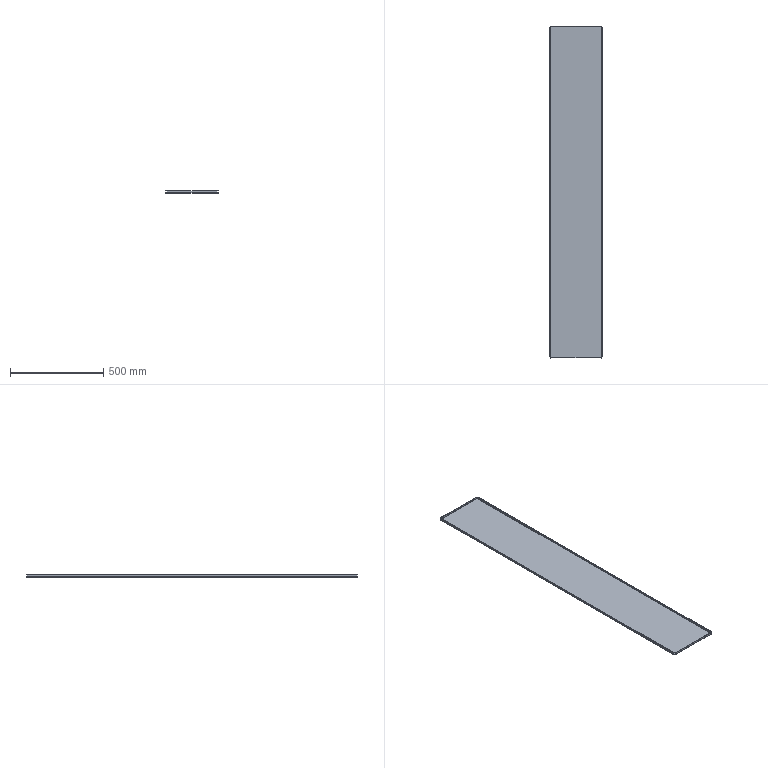Part | SolidWorks | features BaseBody 1 | 1 solid | 50 faces | box 282 x 1776 x 12 mm | volume 1339606 mm3 | plane 42 | cylinder 8 | commonest cylinder face diameters 1.473 x4 6.473 x4
STEP:
#1=CARTESIAN_POINT('',(-134.,885.5,9.5));
#2=VERTEX_POINT('',#1);
#3=CARTESIAN_POINT('',(134.,885.5,9.5));
#4=VERTEX_POINT('',#3);
#5=CARTESIAN_POINT('',(134.,885.5,9.5));
#6=DIRECTION('',(1.,0.,0.));
#7=VECTOR('',#6,1000.);
#8=LINE('',#5,#7);
#9=EDGE_CURVE('',#2,#4,#8,.T.);
#10=ORIENTED_EDGE('',*,*,#9,.T.);
#11=CARTESIAN_POINT('',(134.,888.,9.5));
#12=VERTEX_POINT('',#11);
#13=CARTESIAN_POINT('',(134.,888.,9.5));
#14=DIRECTION('',(0.,-1.,0.));
#15=VECTOR('',#14,1000.);
#16=LINE('',#13,#15);
#17=EDGE_CURVE('',#12,#4,#16,.T.);
#18=ORIENTED_EDGE('',*,*,#17,.F.);
#19=CARTESIAN_POINT('',(-134.,888.,9.5));
#20=VERTEX_POINT('',#19);
#21=CARTESIAN_POINT('',(0.,888.,9.5));
#22=DIRECTION('',(1.,0.,0.));
#23=VECTOR('',#22,1000.);
#24=LINE('',#21,#23);
#25=EDGE_CURVE('',#20,#12,#24,.T.);
#26=ORIENTED_EDGE('',*,*,#25,.F.);
#27=CARTESIAN_POINT('',(-134.,888.,9.5));
#28=DIRECTION('',(0.,-1.,0.));
#29=VECTOR('',#28,1000.);
#30=LINE('',#27,#29);
#31=EDGE_CURVE('',#20,#2,#30,.T.);
#32=ORIENTED_EDGE('',*,*,#31,.T.);
#33=EDGE_LOOP('',(#10,#18,#26,#32));
#34=FACE_OUTER_BOUND('',#33,.T.);
#35=CARTESIAN_POINT('',(134.,888.,9.5));
#36=DIRECTION('',(0.,0.,-1.));
#37=DIRECTION('',(0.,-1.,0.));
#38=AXIS2_PLACEMENT_3D('',#35,#36,#37);
#39=PLANE('',#38);
#40=ADVANCED_FACE('',(#34),#39,.F.);
#41=CARTESIAN_POINT('',(-134.,885.5,0.7366));
#42=VERTEX_POINT('',#41);
#43=CARTESIAN_POINT('',(-134.,885.5,9.5));
#44=DIRECTION('',(0.,0.,1.));
#45=VECTOR('',#44,1000.);
#46=LINE('',#43,#45);
#47=EDGE_CURVE('',#42,#2,#46,.T.);
#48=ORIENTED_EDGE('',*,*,#47,.F.);
#49=CARTESIAN_POINT('',(134.,885.5,0.7366));
#50=VERTEX_POINT('',#49);
#51=CARTESIAN_POINT('',(134.,885.5,0.7366));
#52=DIRECTION('',(-1.,0.,0.));
#53=VECTOR('',#52,1000.);
#54=LINE('',#51,#53);
#55=EDGE_CURVE('',#50,#42,#54,.T.);
#56=ORIENTED_EDGE('',*,*,#55,.F.);
#57=CARTESIAN_POINT('',(134.,885.5,0.));
#58=DIRECTION('',(0.,0.,-1.));
#59=VECTOR('',#58,1000.);
#60=LINE('',#57,#59);
#61=EDGE_CURVE('',#4,#50,#60,.T.);
#62=ORIENTED_EDGE('',*,*,#61,.F.);
#63=ORIENTED_EDGE('',*,*,#9,.F.);
#64=EDGE_LOOP('',(#48,#56,#62,#63));
#65=FACE_OUTER_BOUND('',#64,.T.);
#66=CARTESIAN_POINT('',(0.,885.5,0.));
#67=DIRECTION('',(0.,-1.,0.));
#68=DIRECTION('',(0.,0.,-1.));
#69=AXIS2_PLACEMENT_3D('',#66,#67,#68);
#70=PLANE('',#69);
#71=ADVANCED_FACE('',(#65),#70,.T.);
#72=CARTESIAN_POINT('',(-134.,888.,0.7366));
#73=VERTEX_POINT('',#72);
#74=CARTESIAN_POINT('',(134.,888.,0.7366));
#75=VERTEX_POINT('',#74);
#76=CARTESIAN_POINT('',(134.,888.,0.7366));
#77=DIRECTION('',(1.,0.,0.));
#78=VECTOR('',#77,1000.);
#79=LINE('',#76,#78);
#80=EDGE_CURVE('',#73,#75,#79,.T.);
#81=ORIENTED_EDGE('',*,*,#80,.F.);
#82=CARTESIAN_POINT('',(-134.,888.,0.));
#83=DIRECTION('',(0.,0.,1.));
#84=VECTOR('',#83,1000.);
#85=LINE('',#82,#84);
#86=EDGE_CURVE('',#73,#20,#85,.T.);
#87=ORIENTED_EDGE('',*,*,#86,.T.);
#88=ORIENTED_EDGE('',*,*,#25,.T.);
#89=CARTESIAN_POINT('',(134.,888.,0.));
#90=DIRECTION('',(0.,0.,-1.));
#91=VECTOR('',#90,1000.);
#92=LINE('',#89,#91);
#93=EDGE_CURVE('',#12,#75,#92,.T.);
#94=ORIENTED_EDGE('',*,*,#93,.T.);
#95=EDGE_LOOP('',(#81,#87,#88,#94));
#96=FACE_OUTER_BOUND('',#95,.T.);
#97=CARTESIAN_POINT('',(0.,888.,0.));
#98=DIRECTION('',(0.,-1.,0.));
#99=DIRECTION('',(0.,0.,-1.));
#100=AXIS2_PLACEMENT_3D('',#97,#98,#99);
#101=PLANE('',#100);
#102=ADVANCED_FACE('',(#96),#101,.F.);
#103=CARTESIAN_POINT('',(-134.,885.5,0.7366));
#104=DIRECTION('',(0.,1.,0.));
#105=VECTOR('',#104,1000.);
#106=LINE('',#103,#105);
#107=EDGE_CURVE('',#42,#73,#106,.T.);
#108=ORIENTED_EDGE('',*,*,#107,.F.);
#109=ORIENTED_EDGE('',*,*,#47,.T.);
#110=ORIENTED_EDGE('',*,*,#31,.F.);
#111=ORIENTED_EDGE('',*,*,#86,.F.);
#112=EDGE_LOOP('',(#108,#109,#110,#111));
#113=FACE_OUTER_BOUND('',#112,.T.);
#114=CARTESIAN_POINT('',(-134.,888.,9.5));
#115=DIRECTION('',(1.,0.,0.));
#116=DIRECTION('',(0.,1.,0.));
#117=AXIS2_PLACEMENT_3D('',#114,#115,#116);
#118=PLANE('',#117);
#119=ADVANCED_FACE('',(#113),#118,.F.);
#120=CARTESIAN_POINT('',(134.,888.,0.7366));
#121=DIRECTION('',(0.,1.,0.));
#122=VECTOR('',#121,1000.);
#123=LINE('',#120,#122);
#124=EDGE_CURVE('',#50,#75,#123,.T.);
#125=ORIENTED_EDGE('',*,*,#124,.T.);
#126=ORIENTED_EDGE('',*,*,#93,.F.);
#127=ORIENTED_EDGE('',*,*,#17,.T.);
#128=ORIENTED_EDGE('',*,*,#61,.T.);
#129=EDGE_LOOP('',(#125,#126,#127,#128));
#130=FACE_OUTER_BOUND('',#129,.T.);
#131=CARTESIAN_POINT('',(134.,888.,0.));
#132=DIRECTION('',(-1.,0.,0.));
#133=DIRECTION('',(0.,0.,1.));
#134=AXIS2_PLACEMENT_3D('',#131,#132,#133);
#135=PLANE('',#134);
#136=ADVANCED_FACE('',(#130),#135,.F.);
#137=CARTESIAN_POINT('',(-134.,884.763,0.));
#138=VERTEX_POINT('',#137);
#139=CARTESIAN_POINT('',(134.,884.763,0.));
#140=VERTEX_POINT('',#139);
#141=CARTESIAN_POINT('',(-134.,884.763,0.));
#142=DIRECTION('',(1.,0.,0.));
#143=VECTOR('',#142,1000.);
#144=LINE('',#141,#143);
#145=EDGE_CURVE('',#138,#140,#144,.T.);
#146=ORIENTED_EDGE('',*,*,#145,.T.);
#147=CARTESIAN_POINT('',(134.,884.763,0.7366));
#148=DIRECTION('',(1.,0.,0.));
#149=DIRECTION('',(0.,0.,1.));
#150=AXIS2_PLACEMENT_3D('',#147,#148,#149);
#151=CIRCLE('',#150,0.7366);
#152=EDGE_CURVE('',#140,#50,#151,.T.);
#153=ORIENTED_EDGE('',*,*,#152,.T.);
#154=ORIENTED_EDGE('',*,*,#55,.T.);
#155=CARTESIAN_POINT('',(-134.,884.763,0.7366));
#156=DIRECTION('',(-1.,0.,0.));
#157=DIRECTION('',(0.,0.,1.));
#158=AXIS2_PLACEMENT_3D('',#155,#156,#157);
#159=CIRCLE('',#158,0.7366);
#160=EDGE_CURVE('',#42,#138,#159,.T.);
#161=ORIENTED_EDGE('',*,*,#160,.T.);
#162=EDGE_LOOP('',(#146,#153,#154,#161));
#163=FACE_OUTER_BOUND('',#162,.T.);
#164=CARTESIAN_POINT('',(-134.,884.763,0.7366));
#165=DIRECTION('',(-1.,0.,0.));
#166=DIRECTION('',(0.,1.,0.));
#167=AXIS2_PLACEMENT_3D('',#164,#165,#166);
#168=CYLINDRICAL_SURFACE('',#167,0.7366);
#169=ADVANCED_FACE('',(#163),#168,.F.);
#170=CARTESIAN_POINT('',(-134.,884.763,-2.5));
#171=VERTEX_POINT('',#170);
#172=CARTESIAN_POINT('',(134.,884.763,-2.5));
#173=VERTEX_POINT('',#172);
#174=CARTESIAN_POINT('',(-134.,884.763,-2.5));
#175=DIRECTION('',(1.,0.,0.));
#176=VECTOR('',#175,1000.);
#177=LINE('',#174,#176);
#178=EDGE_CURVE('',#171,#173,#177,.T.);
#179=ORIENTED_EDGE('',*,*,#178,.F.);
#180=CARTESIAN_POINT('',(-134.,887.915,0.));
#181=VERTEX_POINT('',#180);
#182=CARTESIAN_POINT('',(-134.,884.763,0.7366));
#183=DIRECTION('',(-1.,0.,0.));
#184=DIRECTION('',(0.,0.,1.));
#185=AXIS2_PLACEMENT_3D('',#182,#183,#184);
#186=CIRCLE('',#185,3.237);
#187=EDGE_CURVE('',#181,#171,#186,.T.);
#188=ORIENTED_EDGE('',*,*,#187,.F.);
#189=CARTESIAN_POINT('',(-134.,884.763,0.7366));
#190=DIRECTION('',(-1.,0.,0.));
#191=DIRECTION('',(0.,0.,1.));
#192=AXIS2_PLACEMENT_3D('',#189,#190,#191);
#193=CIRCLE('',#192,3.237);
#194=EDGE_CURVE('',#73,#181,#193,.T.);
#195=ORIENTED_EDGE('',*,*,#194,.F.);
#196=ORIENTED_EDGE('',*,*,#80,.T.);
#197=CARTESIAN_POINT('',(134.,887.915,0.));
#198=VERTEX_POINT('',#197);
#199=CARTESIAN_POINT('',(134.,884.763,0.7366));
#200=DIRECTION('',(1.,0.,0.));
#201=DIRECTION('',(0.,0.,1.));
#202=AXIS2_PLACEMENT_3D('',#199,#200,#201);
#203=CIRCLE('',#202,3.237);
#204=EDGE_CURVE('',#198,#75,#203,.T.);
#205=ORIENTED_EDGE('',*,*,#204,.F.);
#206=CARTESIAN_POINT('',(134.,884.763,0.7366));
#207=DIRECTION('',(1.,0.,0.));
#208=DIRECTION('',(0.,0.,1.));
#209=AXIS2_PLACEMENT_3D('',#206,#207,#208);
#210=CIRCLE('',#209,3.237);
#211=EDGE_CURVE('',#173,#198,#210,.T.);
#212=ORIENTED_EDGE('',*,*,#211,.F.);
#213=EDGE_LOOP('',(#179,#188,#195,#196,#205,#212));
#214=FACE_OUTER_BOUND('',#213,.T.);
#215=CARTESIAN_POINT('',(-134.,884.763,0.7366));
#216=DIRECTION('',(-1.,0.,0.));
#217=DIRECTION('',(0.,1.,0.));
#218=AXIS2_PLACEMENT_3D('',#215,#216,#217);
#219=CYLINDRICAL_SURFACE('',#218,3.237);
#220=ADVANCED_FACE('',(#214),#219,.T.);
#221=ORIENTED_EDGE('',*,*,#194,.T.);
#222=CARTESIAN_POINT('',(-134.,888.,0.));
#223=DIRECTION('',(0.,-1.,0.));
#224=VECTOR('',#223,1000.);
#225=LINE('',#222,#224);
#226=EDGE_CURVE('',#181,#138,#225,.T.);
#227=ORIENTED_EDGE('',*,*,#226,.T.);
#228=ORIENTED_EDGE('',*,*,#160,.F.);
#229=ORIENTED_EDGE('',*,*,#107,.T.);
#230=EDGE_LOOP('',(#221,#227,#228,#229));
#231=FACE_OUTER_BOUND('',#230,.T.);
#232=CARTESIAN_POINT('',(-134.,884.763,0.7366));
#233=DIRECTION('',(1.,0.,0.));
#234=DIRECTION('',(0.,1.,0.));
#235=AXIS2_PLACEMENT_3D('',#232,#233,#234);
#236=PLANE('',#235);
#237=ADVANCED_FACE('',(#231),#236,.F.);
#238=ORIENTED_EDGE('',*,*,#152,.F.);
#239=CARTESIAN_POINT('',(134.,884.763,0.));
#240=DIRECTION('',(0.,1.,0.));
#241=VECTOR('',#240,1000.);
#242=LINE('',#239,#241);
#243=EDGE_CURVE('',#140,#198,#242,.T.);
#244=ORIENTED_EDGE('',*,*,#243,.T.);
#245=ORIENTED_EDGE('',*,*,#204,.T.);
#246=ORIENTED_EDGE('',*,*,#124,.F.);
#247=EDGE_LOOP('',(#238,#244,#245,#246));
#248=FACE_OUTER_BOUND('',#247,.T.);
#249=CARTESIAN_POINT('',(134.,884.763,0.7366));
#250=DIRECTION('',(1.,0.,0.));
#251=DIRECTION('',(0.,1.,0.));
#252=AXIS2_PLACEMENT_3D('',#249,#250,#251);
#253=PLANE('',#252);
#254=ADVANCED_FACE('',(#248),#253,.T.);
#255=CARTESIAN_POINT('',(138.5,881.,9.5));
#256=VERTEX_POINT('',#255);
#257=CARTESIAN_POINT('',(138.5,-881.,9.5));
#258=VERTEX_POINT('',#257);
#259=CARTESIAN_POINT('',(138.5,-881.,9.5));
#260=DIRECTION('',(0.,-1.,0.));
#261=VECTOR('',#260,1000.);
#262=LINE('',#259,#261);
#263=EDGE_CURVE('',#256,#258,#262,.T.);
#264=ORIENTED_EDGE('',*,*,#263,.T.);
#265=CARTESIAN_POINT('',(141.,-881.,9.5));
#266=VERTEX_POINT('',#265);
#267=CARTESIAN_POINT('',(141.,-881.,9.5));
#268=DIRECTION('',(-1.,0.,0.));
#269=VECTOR('',#268,1000.);
#270=LINE('',#267,#269);
#271=EDGE_CURVE('',#266,#258,#270,.T.);
#272=ORIENTED_EDGE('',*,*,#271,.F.);
#273=CARTESIAN_POINT('',(141.,881.,9.5));
#274=VERTEX_POINT('',#273);
#275=CARTESIAN_POINT('',(141.,0.,9.5));
#276=DIRECTION('',(0.,-1.,0.));
#277=VECTOR('',#276,1000.);
#278=LINE('',#275,#277);
#279=EDGE_CURVE('',#274,#266,#278,.T.);
#280=ORIENTED_EDGE('',*,*,#279,.F.);
#281=CARTESIAN_POINT('',(141.,881.,9.5));
#282=DIRECTION('',(-1.,0.,0.));
#283=VECTOR('',#282,1000.);
#284=LINE('',#281,#283);
#285=EDGE_CURVE('',#274,#256,#284,.T.);
#286=ORIENTED_EDGE('',*,*,#285,.T.);
#287=EDGE_LOOP('',(#264,#272,#280,#286));
#288=FACE_OUTER_BOUND('',#287,.T.);
#289=CARTESIAN_POINT('',(141.,-881.,9.5));
#290=DIRECTION('',(0.,0.,-1.));
#291=DIRECTION('',(-1.,0.,0.));
#292=AXIS2_PLACEMENT_3D('',#289,#290,#291);
#293=PLANE('',#292);
#294=ADVANCED_FACE('',(#288),#293,.F.);
#295=CARTESIAN_POINT('',(138.5,881.,0.7366));
#296=VERTEX_POINT('',#295);
#297=CARTESIAN_POINT('',(138.5,881.,9.5));
#298=DIRECTION('',(0.,0.,1.));
#299=VECTOR('',#298,1000.);
#300=LINE('',#297,#299);
#301=EDGE_CURVE('',#296,#256,#300,.T.);
#302=ORIENTED_EDGE('',*,*,#301,.F.);
#303=CARTESIAN_POINT('',(138.5,-881.,0.7366));
#304=VERTEX_POINT('',#303);
#305=CARTESIAN_POINT('',(138.5,-881.,0.7366));
#306=DIRECTION('',(0.,1.,0.));
#307=VECTOR('',#306,1000.);
#308=LINE('',#305,#307);
#309=EDGE_CURVE('',#304,#296,#308,.T.);
#310=ORIENTED_EDGE('',*,*,#309,.F.);
#311=CARTESIAN_POINT('',(138.5,-881.,0.));
#312=DIRECTION('',(0.,0.,-1.));
#313=VECTOR('',#312,1000.);
#314=LINE('',#311,#313);
#315=EDGE_CURVE('',#258,#304,#314,.T.);
#316=ORIENTED_EDGE('',*,*,#315,.F.);
#317=ORIENTED_EDGE('',*,*,#263,.F.);
#318=EDGE_LOOP('',(#302,#310,#316,#317));
#319=FACE_OUTER_BOUND('',#318,.T.);
#320=CARTESIAN_POINT('',(138.5,0.,0.));
#321=DIRECTION('',(-1.,0.,0.));
#322=DIRECTION('',(0.,1.,0.));
#323=AXIS2_PLACEMENT_3D('',#320,#321,#322);
#324=PLANE('',#323);
#325=ADVANCED_FACE('',(#319),#324,.T.);
#326=CARTESIAN_POINT('',(141.,881.,0.7366));
#327=VERTEX_POINT('',#326);
#328=CARTESIAN_POINT('',(141.,-881.,0.7366));
#329=VERTEX_POINT('',#328);
#330=CARTESIAN_POINT('',(141.,-881.,0.7366));
#331=DIRECTION('',(0.,-1.,0.));
#332=VECTOR('',#331,1000.);
#333=LINE('',#330,#332);
#334=EDGE_CURVE('',#327,#329,#333,.T.);
#335=ORIENTED_EDGE('',*,*,#334,.F.);
#336=CARTESIAN_POINT('',(141.,881.,0.));
#337=DIRECTION('',(0.,0.,1.));
#338=VECTOR('',#337,1000.);
#339=LINE('',#336,#338);
#340=EDGE_CURVE('',#327,#274,#339,.T.);
#341=ORIENTED_EDGE('',*,*,#340,.T.);
#342=ORIENTED_EDGE('',*,*,#279,.T.);
#343=CARTESIAN_POINT('',(141.,-881.,0.));
#344=DIRECTION('',(0.,0.,-1.));
#345=VECTOR('',#344,1000.);
#346=LINE('',#343,#345);
#347=EDGE_CURVE('',#266,#329,#346,.T.);
#348=ORIENTED_EDGE('',*,*,#347,.T.);
#349=EDGE_LOOP('',(#335,#341,#342,#348));
#350=FACE_OUTER_BOUND('',#349,.T.);
#351=CARTESIAN_POINT('',(141.,0.,0.));
#352=DIRECTION('',(-1.,0.,0.));
#353=DIRECTION('',(0.,1.,0.));
#354=AXIS2_PLACEMENT_3D('',#351,#352,#353);
#355=PLANE('',#354);
#356=ADVANCED_FACE('',(#350),#355,.F.);
#357=CARTESIAN_POINT('',(138.5,881.,0.7366));
#358=DIRECTION('',(1.,0.,0.));
#359=VECTOR('',#358,1000.);
#360=LINE('',#357,#359);
#361=EDGE_CURVE('',#296,#327,#360,.T.);
#362=ORIENTED_EDGE('',*,*,#361,.F.);
#363=ORIENTED_EDGE('',*,*,#301,.T.);
#364=ORIENTED_EDGE('',*,*,#285,.F.);
#365=ORIENTED_EDGE('',*,*,#340,.F.);
#366=EDGE_LOOP('',(#362,#363,#364,#365));
#367=FACE_OUTER_BOUND('',#366,.T.);
#368=CARTESIAN_POINT('',(141.,881.,9.5));
#369=DIRECTION('',(0.,-1.,0.));
#370=DIRECTION('',(0.,0.,-1.));
#371=AXIS2_PLACEMENT_3D('',#368,#369,#370);
#372=PLANE('',#371);
#373=ADVANCED_FACE('',(#367),#372,.F.);
#374=CARTESIAN_POINT('',(141.,-881.,0.7366));
#375=DIRECTION('',(1.,0.,0.));
#376=VECTOR('',#375,1000.);
#377=LINE('',#374,#376);
#378=EDGE_CURVE('',#304,#329,#377,.T.);
#379=ORIENTED_EDGE('',*,*,#378,.T.);
#380=ORIENTED_EDGE('',*,*,#347,.F.);
#381=ORIENTED_EDGE('',*,*,#271,.T.);
#382=ORIENTED_EDGE('',*,*,#315,.T.);
#383=EDGE_LOOP('',(#379,#380,#381,#382));
#384=FACE_OUTER_BOUND('',#383,.T.);
#385=CARTESIAN_POINT('',(141.,-881.,0.));
#386=DIRECTION('',(0.,1.,0.));
#387=DIRECTION('',(0.,0.,-1.));
#388=AXIS2_PLACEMENT_3D('',#385,#386,#387);
#389=PLANE('',#388);
#390=ADVANCED_FACE('',(#384),#389,.F.);
#391=CARTESIAN_POINT('',(137.763,881.,0.));
#392=VERTEX_POINT('',#391);
#393=CARTESIAN_POINT('',(137.763,-881.,0.));
#394=VERTEX_POINT('',#393);
#395=CARTESIAN_POINT('',(137.763,881.,0.));
#396=DIRECTION('',(0.,-1.,0.));
#397=VECTOR('',#396,1000.);
#398=LINE('',#395,#397);
#399=EDGE_CURVE('',#392,#394,#398,.T.);
#400=ORIENTED_EDGE('',*,*,#399,.T.);
#401=CARTESIAN_POINT('',(137.763,-881.,0.7366));
#402=DIRECTION('',(0.,-1.,0.));
#403=DIRECTION('',(0.,0.,1.));
#404=AXIS2_PLACEMENT_3D('',#401,#402,#403);
#405=CIRCLE('',#404,0.7366);
#406=EDGE_CURVE('',#394,#304,#405,.T.);
#407=ORIENTED_EDGE('',*,*,#406,.T.);
#408=ORIENTED_EDGE('',*,*,#309,.T.);
#409=CARTESIAN_POINT('',(137.763,881.,0.7366));
#410=DIRECTION('',(0.,1.,0.));
#411=DIRECTION('',(0.,0.,1.));
#412=AXIS2_PLACEMENT_3D('',#409,#410,#411);
#413=CIRCLE('',#412,0.7366);
#414=EDGE_CURVE('',#296,#392,#413,.T.);
#415=ORIENTED_EDGE('',*,*,#414,.T.);
#416=EDGE_LOOP('',(#400,#407,#408,#415));
#417=FACE_OUTER_BOUND('',#416,.T.);
#418=CARTESIAN_POINT('',(137.763,881.,0.7366));
#419=DIRECTION('',(0.,1.,0.));
#420=DIRECTION('',(1.,0.,0.));
#421=AXIS2_PLACEMENT_3D('',#418,#419,#420);
#422=CYLINDRICAL_SURFACE('',#421,0.7366);
#423=ADVANCED_FACE('',(#417),#422,.F.);
#424=CARTESIAN_POINT('',(137.763,881.,-2.5));
#425=VERTEX_POINT('',#424);
#426=CARTESIAN_POINT('',(137.763,-881.,-2.5));
#427=VERTEX_POINT('',#426);
#428=CARTESIAN_POINT('',(137.763,881.,-2.5));
#429=DIRECTION('',(0.,-1.,0.));
#430=VECTOR('',#429,1000.);
#431=LINE('',#428,#430);
#432=EDGE_CURVE('',#425,#427,#431,.T.);
#433=ORIENTED_EDGE('',*,*,#432,.F.);
#434=CARTESIAN_POINT('',(140.915,881.,0.));
#435=VERTEX_POINT('',#434);
#436=CARTESIAN_POINT('',(137.763,881.,0.7366));
#437=DIRECTION('',(0.,1.,0.));
#438=DIRECTION('',(0.,0.,1.));
#439=AXIS2_PLACEMENT_3D('',#436,#437,#438);
#440=CIRCLE('',#439,3.237);
#441=EDGE_CURVE('',#435,#425,#440,.T.);
#442=ORIENTED_EDGE('',*,*,#441,.F.);
#443=CARTESIAN_POINT('',(137.763,881.,0.7366));
#444=DIRECTION('',(0.,1.,0.));
#445=DIRECTION('',(0.,0.,1.));
#446=AXIS2_PLACEMENT_3D('',#443,#444,#445);
#447=CIRCLE('',#446,3.237);
#448=EDGE_CURVE('',#327,#435,#447,.T.);
#449=ORIENTED_EDGE('',*,*,#448,.F.);
#450=ORIENTED_EDGE('',*,*,#334,.T.);
#451=CARTESIAN_POINT('',(140.915,-881.,0.));
#452=VERTEX_POINT('',#451);
#453=CARTESIAN_POINT('',(137.763,-881.,0.7366));
#454=DIRECTION('',(0.,-1.,0.));
#455=DIRECTION('',(0.,0.,1.));
#456=AXIS2_PLACEMENT_3D('',#453,#454,#455);
#457=CIRCLE('',#456,3.237);
#458=EDGE_CURVE('',#452,#329,#457,.T.);
#459=ORIENTED_EDGE('',*,*,#458,.F.);
#460=CARTESIAN_POINT('',(137.763,-881.,0.7366));
#461=DIRECTION('',(0.,-1.,0.));
#462=DIRECTION('',(0.,0.,1.));
#463=AXIS2_PLACEMENT_3D('',#460,#461,#462);
#464=CIRCLE('',#463,3.237);
#465=EDGE_CURVE('',#427,#452,#464,.T.);
#466=ORIENTED_EDGE('',*,*,#465,.F.);
#467=EDGE_LOOP('',(#433,#442,#449,#450,#459,#466));
#468=FACE_OUTER_BOUND('',#467,.T.);
#469=CARTESIAN_POINT('',(137.763,881.,0.7366));
#470=DIRECTION('',(0.,1.,0.));
#471=DIRECTION('',(1.,0.,0.));
#472=AXIS2_PLACEMENT_3D('',#469,#470,#471);
#473=CYLINDRICAL_SURFACE('',#472,3.237);
#474=ADVANCED_FACE('',(#468),#473,.T.);
#475=ORIENTED_EDGE('',*,*,#448,.T.);
#476=CARTESIAN_POINT('',(141.,881.,0.));
#477=DIRECTION('',(-1.,0.,0.));
#478=VECTOR('',#477,1000.);
#479=LINE('',#476,#478);
#480=EDGE_CURVE('',#435,#392,#479,.T.);
#481=ORIENTED_EDGE('',*,*,#480,.T.);
#482=ORIENTED_EDGE('',*,*,#414,.F.);
#483=ORIENTED_EDGE('',*,*,#361,.T.);
#484=EDGE_LOOP('',(#475,#481,#482,#483));
#485=FACE_OUTER_BOUND('',#484,.T.);
#486=CARTESIAN_POINT('',(137.763,881.,0.7366));
#487=DIRECTION('',(0.,-1.,0.));
#488=DIRECTION('',(0.,0.,-1.));
#489=AXIS2_PLACEMENT_3D('',#486,#487,#488);
#490=PLANE('',#489);
#491=ADVANCED_FACE('',(#485),#490,.F.);
#492=ORIENTED_EDGE('',*,*,#406,.F.);
#493=CARTESIAN_POINT('',(137.763,-881.,0.));
#494=DIRECTION('',(1.,0.,0.));
#495=VECTOR('',#494,1000.);
#496=LINE('',#493,#495);
#497=EDGE_CURVE('',#394,#452,#496,.T.);
#498=ORIENTED_EDGE('',*,*,#497,.T.);
#499=ORIENTED_EDGE('',*,*,#458,.T.);
#500=ORIENTED_EDGE('',*,*,#378,.F.);
#501=EDGE_LOOP('',(#492,#498,#499,#500));
#502=FACE_OUTER_BOUND('',#501,.T.);
#503=CARTESIAN_POINT('',(137.763,-881.,0.7366));
#504=DIRECTION('',(0.,-1.,0.));
#505=DIRECTION('',(0.,0.,-1.));
#506=AXIS2_PLACEMENT_3D('',#503,#504,#505);
#507=PLANE('',#506);
#508=ADVANCED_FACE('',(#502),#507,.T.);
#509=CARTESIAN_POINT('',(134.,-885.5,9.5));
#510=VERTEX_POINT('',#509);
#511=CARTESIAN_POINT('',(-134.,-885.5,9.5));
#512=VERTEX_POINT('',#511);
#513=CARTESIAN_POINT('',(-134.,-885.5,9.5));
#514=DIRECTION('',(-1.,0.,0.));
#515=VECTOR('',#514,1000.);
#516=LINE('',#513,#515);
#517=EDGE_CURVE('',#510,#512,#516,.T.);
#518=ORIENTED_EDGE('',*,*,#517,.T.);
#519=CARTESIAN_POINT('',(-134.,-888.,9.5));
#520=VERTEX_POINT('',#519);
#521=CARTESIAN_POINT('',(-134.,-888.,9.5));
#522=DIRECTION('',(0.,1.,0.));
#523=VECTOR('',#522,1000.);
#524=LINE('',#521,#523);
#525=EDGE_CURVE('',#520,#512,#524,.T.);
#526=ORIENTED_EDGE('',*,*,#525,.F.);
#527=CARTESIAN_POINT('',(134.,-888.,9.5));
#528=VERTEX_POINT('',#527);
#529=CARTESIAN_POINT('',(0.,-888.,9.5));
#530=DIRECTION('',(-1.,0.,0.));
#531=VECTOR('',#530,1000.);
#532=LINE('',#529,#531);
#533=EDGE_CURVE('',#528,#520,#532,.T.);
#534=ORIENTED_EDGE('',*,*,#533,.F.);
#535=CARTESIAN_POINT('',(134.,-888.,9.5));
#536=DIRECTION('',(0.,1.,0.));
#537=VECTOR('',#536,1000.);
#538=LINE('',#535,#537);
#539=EDGE_CURVE('',#528,#510,#538,.T.);
#540=ORIENTED_EDGE('',*,*,#539,.T.);
#541=EDGE_LOOP('',(#518,#526,#534,#540));
#542=FACE_OUTER_BOUND('',#541,.T.);
#543=CARTESIAN_POINT('',(-134.,-888.,9.5));
#544=DIRECTION('',(0.,0.,-1.));
#545=DIRECTION('',(-1.,0.,0.));
#546=AXIS2_PLACEMENT_3D('',#543,#544,#545);
#547=PLANE('',#546);
#548=ADVANCED_FACE('',(#542),#547,.F.);
#549=CARTESIAN_POINT('',(134.,-885.5,0.7366));
#550=VERTEX_POINT('',#549);
#551=CARTESIAN_POINT('',(134.,-885.5,9.5));
#552=DIRECTION('',(0.,0.,1.));
#553=VECTOR('',#552,1000.);
#554=LINE('',#551,#553);
#555=EDGE_CURVE('',#550,#510,#554,.T.);
#556=ORIENTED_EDGE('',*,*,#555,.F.);
#557=CARTESIAN_POINT('',(-134.,-885.5,0.7366));
#558=VERTEX_POINT('',#557);
#559=CARTESIAN_POINT('',(-134.,-885.5,0.7366));
#560=DIRECTION('',(1.,0.,0.));
#561=VECTOR('',#560,1000.);
#562=LINE('',#559,#561);
#563=EDGE_CURVE('',#558,#550,#562,.T.);
#564=ORIENTED_EDGE('',*,*,#563,.F.);
#565=CARTESIAN_POINT('',(-134.,-885.5,0.));
#566=DIRECTION('',(0.,0.,-1.));
#567=VECTOR('',#566,1000.);
#568=LINE('',#565,#567);
#569=EDGE_CURVE('',#512,#558,#568,.T.);
#570=ORIENTED_EDGE('',*,*,#569,.F.);
#571=ORIENTED_EDGE('',*,*,#517,.F.);
#572=EDGE_LOOP('',(#556,#564,#570,#571));
#573=FACE_OUTER_BOUND('',#572,.T.);
#574=CARTESIAN_POINT('',(0.,-885.5,0.));
#575=DIRECTION('',(0.,1.,0.));
#576=DIRECTION('',(1.,0.,0.));
#577=AXIS2_PLACEMENT_3D('',#574,#575,#576);
#578=PLANE('',#577);
#579=ADVANCED_FACE('',(#573),#578,.T.);
#580=CARTESIAN_POINT('',(134.,-888.,0.7366));
#581=VERTEX_POINT('',#580);
#582=CARTESIAN_POINT('',(-134.,-888.,0.7366));
#583=VERTEX_POINT('',#582);
#584=CARTESIAN_POINT('',(-134.,-888.,0.7366));
#585=DIRECTION('',(-1.,0.,0.));
#586=VECTOR('',#585,1000.);
#587=LINE('',#584,#586);
#588=EDGE_CURVE('',#581,#583,#587,.T.);
#589=ORIENTED_EDGE('',*,*,#588,.F.);
#590=CARTESIAN_POINT('',(134.,-888.,0.));
#591=DIRECTION('',(0.,0.,1.));
#592=VECTOR('',#591,1000.);
#593=LINE('',#590,#592);
#594=EDGE_CURVE('',#581,#528,#593,.T.);
#595=ORIENTED_EDGE('',*,*,#594,.T.);
#596=ORIENTED_EDGE('',*,*,#533,.T.);
#597=CARTESIAN_POINT('',(-134.,-888.,0.));
#598=DIRECTION('',(0.,0.,-1.));
#599=VECTOR('',#598,1000.);
#600=LINE('',#597,#599);
#601=EDGE_CURVE('',#520,#583,#600,.T.);
#602=ORIENTED_EDGE('',*,*,#601,.T.);
#603=EDGE_LOOP('',(#589,#595,#596,#602));
#604=FACE_OUTER_BOUND('',#603,.T.);
#605=CARTESIAN_POINT('',(0.,-888.,0.));
#606=DIRECTION('',(0.,1.,0.));
#607=DIRECTION('',(1.,0.,0.));
#608=AXIS2_PLACEMENT_3D('',#605,#606,#607);
#609=PLANE('',#608);
#610=ADVANCED_FACE('',(#604),#609,.F.);
#611=CARTESIAN_POINT('',(134.,-885.5,0.7366));
#612=DIRECTION('',(0.,-1.,0.));
#613=VECTOR('',#612,1000.);
#614=LINE('',#611,#613);
#615=EDGE_CURVE('',#550,#581,#614,.T.);
#616=ORIENTED_EDGE('',*,*,#615,.F.);
#617=ORIENTED_EDGE('',*,*,#555,.T.);
#618=ORIENTED_EDGE('',*,*,#539,.F.);
#619=ORIENTED_EDGE('',*,*,#594,.F.);
#620=EDGE_LOOP('',(#616,#617,#618,#619));
#621=FACE_OUTER_BOUND('',#620,.T.);
#622=CARTESIAN_POINT('',(134.,-888.,9.5));
#623=DIRECTION('',(-1.,0.,0.));
#624=DIRECTION('',(0.,0.,1.));
#625=AXIS2_PLACEMENT_3D('',#622,#623,#624);
#626=PLANE('',#625);
#627=ADVANCED_FACE('',(#621),#626,.F.);
#628=CARTESIAN_POINT('',(-134.,-888.,0.7366));
#629=DIRECTION('',(0.,-1.,0.));
#630=VECTOR('',#629,1000.);
#631=LINE('',#628,#630);
#632=EDGE_CURVE('',#558,#583,#631,.T.);
#633=ORIENTED_EDGE('',*,*,#632,.T.);
#634=ORIENTED_EDGE('',*,*,#601,.F.);
#635=ORIENTED_EDGE('',*,*,#525,.T.);
#636=ORIENTED_EDGE('',*,*,#569,.T.);
#637=EDGE_LOOP('',(#633,#634,#635,#636));
#638=FACE_OUTER_BOUND('',#637,.T.);
#639=CARTESIAN_POINT('',(-134.,-888.,0.));
#640=DIRECTION('',(1.,0.,0.));
#641=DIRECTION('',(0.,1.,0.));
#642=AXIS2_PLACEMENT_3D('',#639,#640,#641);
#643=PLANE('',#642);
#644=ADVANCED_FACE('',(#638),#643,.F.);
#645=CARTESIAN_POINT('',(134.,-884.763,0.));
#646=VERTEX_POINT('',#645);
#647=CARTESIAN_POINT('',(-134.,-884.763,0.));
#648=VERTEX_POINT('',#647);
#649=CARTESIAN_POINT('',(134.,-884.763,0.));
#650=DIRECTION('',(-1.,0.,0.));
#651=VECTOR('',#650,1000.);
#652=LINE('',#649,#651);
#653=EDGE_CURVE('',#646,#648,#652,.T.);
#654=ORIENTED_EDGE('',*,*,#653,.T.);
#655=CARTESIAN_POINT('',(-134.,-884.763,0.7366));
#656=DIRECTION('',(-1.,0.,0.));
#657=DIRECTION('',(0.,0.,-1.));
#658=AXIS2_PLACEMENT_3D('',#655,#656,#657);
#659=CIRCLE('',#658,0.7366);
#660=EDGE_CURVE('',#648,#558,#659,.T.);
#661=ORIENTED_EDGE('',*,*,#660,.T.);
#662=ORIENTED_EDGE('',*,*,#563,.T.);
#663=CARTESIAN_POINT('',(134.,-884.763,0.7366));
#664=DIRECTION('',(1.,0.,0.));
#665=DIRECTION('',(0.,0.,-1.));
#666=AXIS2_PLACEMENT_3D('',#663,#664,#665);
#667=CIRCLE('',#666,0.7366);
#668=EDGE_CURVE('',#550,#646,#667,.T.);
#669=ORIENTED_EDGE('',*,*,#668,.T.);
#670=EDGE_LOOP('',(#654,#661,#662,#669));
#671=FACE_OUTER_BOUND('',#670,.T.);
#672=CARTESIAN_POINT('',(134.,-884.763,0.7366));
#673=DIRECTION('',(1.,0.,0.));
#674=DIRECTION('',(0.,-1.,0.));
#675=AXIS2_PLACEMENT_3D('',#672,#673,#674);
#676=CYLINDRICAL_SURFACE('',#675,0.7366);
#677=ADVANCED_FACE('',(#671),#676,.F.);
#678=CARTESIAN_POINT('',(134.,-884.763,-2.5));
#679=VERTEX_POINT('',#678);
#680=CARTESIAN_POINT('',(-134.,-884.763,-2.5));
#681=VERTEX_POINT('',#680);
#682=CARTESIAN_POINT('',(134.,-884.763,-2.5));
#683=DIRECTION('',(-1.,0.,0.));
#684=VECTOR('',#683,1000.);
#685=LINE('',#682,#684);
#686=EDGE_CURVE('',#679,#681,#685,.T.);
#687=ORIENTED_EDGE('',*,*,#686,.F.);
#688=CARTESIAN_POINT('',(134.,-887.915,0.));
#689=VERTEX_POINT('',#688);
#690=CARTESIAN_POINT('',(134.,-884.763,0.7366));
#691=DIRECTION('',(1.,0.,0.));
#692=DIRECTION('',(0.,0.,-1.));
#693=AXIS2_PLACEMENT_3D('',#690,#691,#692);
#694=CIRCLE('',#693,3.237);
#695=EDGE_CURVE('',#689,#679,#694,.T.);
#696=ORIENTED_EDGE('',*,*,#695,.F.);
#697=CARTESIAN_POINT('',(134.,-884.763,0.7366));
#698=DIRECTION('',(1.,0.,0.));
#699=DIRECTION('',(0.,0.,-1.));
#700=AXIS2_PLACEMENT_3D('',#697,#698,#699);
#701=CIRCLE('',#700,3.237);
#702=EDGE_CURVE('',#581,#689,#701,.T.);
#703=ORIENTED_EDGE('',*,*,#702,.F.);
#704=ORIENTED_EDGE('',*,*,#588,.T.);
#705=CARTESIAN_POINT('',(-134.,-887.915,0.));
#706=VERTEX_POINT('',#705);
#707=CARTESIAN_POINT('',(-134.,-884.763,0.7366));
#708=DIRECTION('',(-1.,0.,0.));
#709=DIRECTION('',(0.,0.,-1.));
#710=AXIS2_PLACEMENT_3D('',#707,#708,#709);
#711=CIRCLE('',#710,3.237);
#712=EDGE_CURVE('',#706,#583,#711,.T.);
#713=ORIENTED_EDGE('',*,*,#712,.F.);
#714=CARTESIAN_POINT('',(-134.,-884.763,0.7366));
#715=DIRECTION('',(-1.,0.,0.));
#716=DIRECTION('',(0.,0.,-1.));
#717=AXIS2_PLACEMENT_3D('',#714,#715,#716);
#718=CIRCLE('',#717,3.237);
#719=EDGE_CURVE('',#681,#706,#718,.T.);
#720=ORIENTED_EDGE('',*,*,#719,.F.);
#721=EDGE_LOOP('',(#687,#696,#703,#704,#713,#720));
#722=FACE_OUTER_BOUND('',#721,.T.);
#723=CARTESIAN_POINT('',(134.,-884.763,0.7366));
#724=DIRECTION('',(1.,0.,0.));
#725=DIRECTION('',(0.,-1.,0.));
#726=AXIS2_PLACEMENT_3D('',#723,#724,#725);
#727=CYLINDRICAL_SURFACE('',#726,3.237);
#728=ADVANCED_FACE('',(#722),#727,.T.);
#729=ORIENTED_EDGE('',*,*,#702,.T.);
#730=CARTESIAN_POINT('',(134.,-888.,0.));
#731=DIRECTION('',(0.,1.,0.));
#732=VECTOR('',#731,1000.);
#733=LINE('',#730,#732);
#734=EDGE_CURVE('',#689,#646,#733,.T.);
#735=ORIENTED_EDGE('',*,*,#734,.T.);
#736=ORIENTED_EDGE('',*,*,#668,.F.);
#737=ORIENTED_EDGE('',*,*,#615,.T.);
#738=EDGE_LOOP('',(#729,#735,#736,#737));
#739=FACE_OUTER_BOUND('',#738,.T.);
#740=CARTESIAN_POINT('',(134.,-884.763,0.7366));
#741=DIRECTION('',(-1.,0.,0.));
#742=DIRECTION('',(0.,0.,1.));
#743=AXIS2_PLACEMENT_3D('',#740,#741,#742);
#744=PLANE('',#743);
#745=ADVANCED_FACE('',(#739),#744,.F.);
#746=ORIENTED_EDGE('',*,*,#660,.F.);
#747=CARTESIAN_POINT('',(-134.,-884.763,0.));
#748=DIRECTION('',(0.,-1.,0.));
#749=VECTOR('',#748,1000.);
#750=LINE('',#747,#749);
#751=EDGE_CURVE('',#648,#706,#750,.T.);
#752=ORIENTED_EDGE('',*,*,#751,.T.);
#753=ORIENTED_EDGE('',*,*,#712,.T.);
#754=ORIENTED_EDGE('',*,*,#632,.F.);
#755=EDGE_LOOP('',(#746,#752,#753,#754));
#756=FACE_OUTER_BOUND('',#755,.T.);
#757=CARTESIAN_POINT('',(-134.,-884.763,0.7366));
#758=DIRECTION('',(-1.,0.,0.));
#759=DIRECTION('',(0.,0.,1.));
#760=AXIS2_PLACEMENT_3D('',#757,#758,#759);
#761=PLANE('',#760);
#762=ADVANCED_FACE('',(#756),#761,.T.);
#763=CARTESIAN_POINT('',(-138.5,-881.,9.5));
#764=VERTEX_POINT('',#763);
#765=CARTESIAN_POINT('',(-138.5,881.,9.5));
#766=VERTEX_POINT('',#765);
#767=CARTESIAN_POINT('',(-138.5,881.,9.5));
#768=DIRECTION('',(0.,1.,0.));
#769=VECTOR('',#768,1000.);
#770=LINE('',#767,#769);
#771=EDGE_CURVE('',#764,#766,#770,.T.);
#772=ORIENTED_EDGE('',*,*,#771,.T.);
#773=CARTESIAN_POINT('',(-141.,881.,9.5));
#774=VERTEX_POINT('',#773);
#775=CARTESIAN_POINT('',(-141.,881.,9.5));
#776=DIRECTION('',(1.,0.,0.));
#777=VECTOR('',#776,1000.);
#778=LINE('',#775,#777);
#779=EDGE_CURVE('',#774,#766,#778,.T.);
#780=ORIENTED_EDGE('',*,*,#779,.F.);
#781=CARTESIAN_POINT('',(-141.,-881.,9.5));
#782=VERTEX_POINT('',#781);
#783=CARTESIAN_POINT('',(-141.,0.,9.5));
#784=DIRECTION('',(0.,1.,0.));
#785=VECTOR('',#784,1000.);
#786=LINE('',#783,#785);
#787=EDGE_CURVE('',#782,#774,#786,.T.);
#788=ORIENTED_EDGE('',*,*,#787,.F.);
#789=CARTESIAN_POINT('',(-141.,-881.,9.5));
#790=DIRECTION('',(1.,0.,0.));
#791=VECTOR('',#790,1000.);
#792=LINE('',#789,#791);
#793=EDGE_CURVE('',#782,#764,#792,.T.);
#794=ORIENTED_EDGE('',*,*,#793,.T.);
#795=EDGE_LOOP('',(#772,#780,#788,#794));
#796=FACE_OUTER_BOUND('',#795,.T.);
#797=CARTESIAN_POINT('',(-141.,881.,9.5));
#798=DIRECTION('',(0.,0.,-1.));
#799=DIRECTION('',(0.,-1.,0.));
#800=AXIS2_PLACEMENT_3D('',#797,#798,#799);
#801=PLANE('',#800);
#802=ADVANCED_FACE('',(#796),#801,.F.);
#803=CARTESIAN_POINT('',(-138.5,-881.,0.7366));
#804=VERTEX_POINT('',#803);
#805=CARTESIAN_POINT('',(-138.5,-881.,9.5));
#806=DIRECTION('',(0.,0.,1.));
#807=VECTOR('',#806,1000.);
#808=LINE('',#805,#807);
#809=EDGE_CURVE('',#804,#764,#808,.T.);
#810=ORIENTED_EDGE('',*,*,#809,.F.);
#811=CARTESIAN_POINT('',(-138.5,881.,0.7366));
#812=VERTEX_POINT('',#811);
#813=CARTESIAN_POINT('',(-138.5,881.,0.7366));
#814=DIRECTION('',(0.,-1.,0.));
#815=VECTOR('',#814,1000.);
#816=LINE('',#813,#815);
#817=EDGE_CURVE('',#812,#804,#816,.T.);
#818=ORIENTED_EDGE('',*,*,#817,.F.);
#819=CARTESIAN_POINT('',(-138.5,881.,0.));
#820=DIRECTION('',(0.,0.,-1.));
#821=VECTOR('',#820,1000.);
#822=LINE('',#819,#821);
#823=EDGE_CURVE('',#766,#812,#822,.T.);
#824=ORIENTED_EDGE('',*,*,#823,.F.);
#825=ORIENTED_EDGE('',*,*,#771,.F.);
#826=EDGE_LOOP('',(#810,#818,#824,#825));
#827=FACE_OUTER_BOUND('',#826,.T.);
#828=CARTESIAN_POINT('',(-138.5,0.,0.));
#829=DIRECTION('',(1.,0.,0.));
#830=DIRECTION('',(0.,0.,1.));
#831=AXIS2_PLACEMENT_3D('',#828,#829,#830);
#832=PLANE('',#831);
#833=ADVANCED_FACE('',(#827),#832,.T.);
#834=CARTESIAN_POINT('',(-141.,-881.,0.7366));
#835=VERTEX_POINT('',#834);
#836=CARTESIAN_POINT('',(-141.,881.,0.7366));
#837=VERTEX_POINT('',#836);
#838=CARTESIAN_POINT('',(-141.,881.,0.7366));
#839=DIRECTION('',(0.,1.,0.));
#840=VECTOR('',#839,1000.);
#841=LINE('',#838,#840);
#842=EDGE_CURVE('',#835,#837,#841,.T.);
#843=ORIENTED_EDGE('',*,*,#842,.F.);
#844=CARTESIAN_POINT('',(-141.,-881.,0.));
#845=DIRECTION('',(0.,0.,1.));
#846=VECTOR('',#845,1000.);
#847=LINE('',#844,#846);
#848=EDGE_CURVE('',#835,#782,#847,.T.);
#849=ORIENTED_EDGE('',*,*,#848,.T.);
#850=ORIENTED_EDGE('',*,*,#787,.T.);
#851=CARTESIAN_POINT('',(-141.,881.,0.));
#852=DIRECTION('',(0.,0.,-1.));
#853=VECTOR('',#852,1000.);
#854=LINE('',#851,#853);
#855=EDGE_CURVE('',#774,#837,#854,.T.);
#856=ORIENTED_EDGE('',*,*,#855,.T.);
#857=EDGE_LOOP('',(#843,#849,#850,#856));
#858=FACE_OUTER_BOUND('',#857,.T.);
#859=CARTESIAN_POINT('',(-141.,0.,0.));
#860=DIRECTION('',(1.,0.,0.));
#861=DIRECTION('',(0.,0.,1.));
#862=AXIS2_PLACEMENT_3D('',#859,#860,#861);
#863=PLANE('',#862);
#864=ADVANCED_FACE('',(#858),#863,.F.);
#865=CARTESIAN_POINT('',(-141.,881.,0.7366));
#866=DIRECTION('',(-1.,0.,0.));
#867=VECTOR('',#866,1000.);
#868=LINE('',#865,#867);
#869=EDGE_CURVE('',#812,#837,#868,.T.);
#870=ORIENTED_EDGE('',*,*,#869,.T.);
#871=ORIENTED_EDGE('',*,*,#855,.F.);
#872=ORIENTED_EDGE('',*,*,#779,.T.);
#873=ORIENTED_EDGE('',*,*,#823,.T.);
#874=EDGE_LOOP('',(#870,#871,#872,#873));
#875=FACE_OUTER_BOUND('',#874,.T.);
#876=CARTESIAN_POINT('',(-141.,881.,0.));
#877=DIRECTION('',(0.,-1.,0.));
#878=DIRECTION('',(0.,0.,-1.));
#879=AXIS2_PLACEMENT_3D('',#876,#877,#878);
#880=PLANE('',#879);
#881=ADVANCED_FACE('',(#875),#880,.F.);
#882=CARTESIAN_POINT('',(-138.5,-881.,0.7366));
#883=DIRECTION('',(-1.,0.,0.));
#884=VECTOR('',#883,1000.);
#885=LINE('',#882,#884);
#886=EDGE_CURVE('',#804,#835,#885,.T.);
#887=ORIENTED_EDGE('',*,*,#886,.F.);
#888=ORIENTED_EDGE('',*,*,#809,.T.);
#889=ORIENTED_EDGE('',*,*,#793,.F.);
#890=ORIENTED_EDGE('',*,*,#848,.F.);
#891=EDGE_LOOP('',(#887,#888,#889,#890));
#892=FACE_OUTER_BOUND('',#891,.T.);
#893=CARTESIAN_POINT('',(-141.,-881.,9.5));
#894=DIRECTION('',(0.,1.,0.));
#895=DIRECTION('',(0.,0.,-1.));
#896=AXIS2_PLACEMENT_3D('',#893,#894,#895);
#897=PLANE('',#896);
#898=ADVANCED_FACE('',(#892),#897,.F.);
#899=CARTESIAN_POINT('',(-137.763,-881.,0.));
#900=VERTEX_POINT('',#899);
#901=CARTESIAN_POINT('',(-137.763,881.,0.));
#902=VERTEX_POINT('',#901);
#903=CARTESIAN_POINT('',(-137.763,-881.,0.));
#904=DIRECTION('',(0.,1.,0.));
#905=VECTOR('',#904,1000.);
#906=LINE('',#903,#905);
#907=EDGE_CURVE('',#900,#902,#906,.T.);
#908=ORIENTED_EDGE('',*,*,#907,.T.);
#909=CARTESIAN_POINT('',(-137.763,881.,0.7366));
#910=DIRECTION('',(0.,1.,0.));
#911=DIRECTION('',(0.,0.,-1.));
#912=AXIS2_PLACEMENT_3D('',#909,#910,#911);
#913=CIRCLE('',#912,0.7366);
#914=EDGE_CURVE('',#902,#812,#913,.T.);
#915=ORIENTED_EDGE('',*,*,#914,.T.);
#916=ORIENTED_EDGE('',*,*,#817,.T.);
#917=CARTESIAN_POINT('',(-137.763,-881.,0.7366));
#918=DIRECTION('',(0.,-1.,0.));
#919=DIRECTION('',(0.,0.,-1.));
#920=AXIS2_PLACEMENT_3D('',#917,#918,#919);
#921=CIRCLE('',#920,0.7366);
#922=EDGE_CURVE('',#804,#900,#921,.T.);
#923=ORIENTED_EDGE('',*,*,#922,.T.);
#924=EDGE_LOOP('',(#908,#915,#916,#923));
#925=FACE_OUTER_BOUND('',#924,.T.);
#926=CARTESIAN_POINT('',(-137.763,-881.,0.7366));
#927=DIRECTION('',(0.,-1.,0.));
#928=DIRECTION('',(-1.,0.,0.));
#929=AXIS2_PLACEMENT_3D('',#926,#927,#928);
#930=CYLINDRICAL_SURFACE('',#929,0.7366);
#931=ADVANCED_FACE('',(#925),#930,.F.);
#932=CARTESIAN_POINT('',(-137.763,-881.,-2.5));
#933=VERTEX_POINT('',#932);
#934=CARTESIAN_POINT('',(-137.763,881.,-2.5));
#935=VERTEX_POINT('',#934);
#936=CARTESIAN_POINT('',(-137.763,-881.,-2.5));
#937=DIRECTION('',(0.,1.,0.));
#938=VECTOR('',#937,1000.);
#939=LINE('',#936,#938);
#940=EDGE_CURVE('',#933,#935,#939,.T.);
#941=ORIENTED_EDGE('',*,*,#940,.F.);
#942=CARTESIAN_POINT('',(-140.915,-881.,0.));
#943=VERTEX_POINT('',#942);
#944=CARTESIAN_POINT('',(-137.763,-881.,0.7366));
#945=DIRECTION('',(0.,-1.,0.));
#946=DIRECTION('',(0.,0.,-1.));
#947=AXIS2_PLACEMENT_3D('',#944,#945,#946);
#948=CIRCLE('',#947,3.237);
#949=EDGE_CURVE('',#943,#933,#948,.T.);
#950=ORIENTED_EDGE('',*,*,#949,.F.);
#951=CARTESIAN_POINT('',(-137.763,-881.,0.7366));
#952=DIRECTION('',(0.,-1.,0.));
#953=DIRECTION('',(0.,0.,-1.));
#954=AXIS2_PLACEMENT_3D('',#951,#952,#953);
#955=CIRCLE('',#954,3.237);
#956=EDGE_CURVE('',#835,#943,#955,.T.);
#957=ORIENTED_EDGE('',*,*,#956,.F.);
#958=ORIENTED_EDGE('',*,*,#842,.T.);
#959=CARTESIAN_POINT('',(-140.915,881.,0.));
#960=VERTEX_POINT('',#959);
#961=CARTESIAN_POINT('',(-137.763,881.,0.7366));
#962=DIRECTION('',(0.,1.,0.));
#963=DIRECTION('',(0.,0.,-1.));
#964=AXIS2_PLACEMENT_3D('',#961,#962,#963);
#965=CIRCLE('',#964,3.237);
#966=EDGE_CURVE('',#960,#837,#965,.T.);
#967=ORIENTED_EDGE('',*,*,#966,.F.);
#968=CARTESIAN_POINT('',(-137.763,881.,0.7366));
#969=DIRECTION('',(0.,1.,0.));
#970=DIRECTION('',(0.,0.,-1.));
#971=AXIS2_PLACEMENT_3D('',#968,#969,#970);
#972=CIRCLE('',#971,3.237);
#973=EDGE_CURVE('',#935,#960,#972,.T.);
#974=ORIENTED_EDGE('',*,*,#973,.F.);
#975=EDGE_LOOP('',(#941,#950,#957,#958,#967,#974));
#976=FACE_OUTER_BOUND('',#975,.T.);
#977=CARTESIAN_POINT('',(-137.763,-881.,0.7366));
#978=DIRECTION('',(0.,-1.,0.));
#979=DIRECTION('',(-1.,0.,0.));
#980=AXIS2_PLACEMENT_3D('',#977,#978,#979);
#981=CYLINDRICAL_SURFACE('',#980,3.237);
#982=ADVANCED_FACE('',(#976),#981,.T.);
#983=ORIENTED_EDGE('',*,*,#956,.T.);
#984=CARTESIAN_POINT('',(-141.,-881.,0.));
#985=DIRECTION('',(1.,0.,0.));
#986=VECTOR('',#985,1000.);
#987=LINE('',#984,#986);
#988=EDGE_CURVE('',#943,#900,#987,.T.);
#989=ORIENTED_EDGE('',*,*,#988,.T.);
#990=ORIENTED_EDGE('',*,*,#922,.F.);
#991=ORIENTED_EDGE('',*,*,#886,.T.);
#992=EDGE_LOOP('',(#983,#989,#990,#991));
#993=FACE_OUTER_BOUND('',#992,.T.);
#994=CARTESIAN_POINT('',(-137.763,-881.,0.7366));
#995=DIRECTION('',(0.,1.,0.));
#996=DIRECTION('',(1.,0.,0.));
#997=AXIS2_PLACEMENT_3D('',#994,#995,#996);
#998=PLANE('',#997);
#999=ADVANCED_FACE('',(#993),#998,.F.);
#1000=ORIENTED_EDGE('',*,*,#914,.F.);
#1001=CARTESIAN_POINT('',(-137.763,881.,0.));
#1002=DIRECTION('',(-1.,0.,0.));
#1003=VECTOR('',#1002,1000.);
#1004=LINE('',#1001,#1003);
#1005=EDGE_CURVE('',#902,#960,#1004,.T.);
#1006=ORIENTED_EDGE('',*,*,#1005,.T.);
#1007=ORIENTED_EDGE('',*,*,#966,.T.);
#1008=ORIENTED_EDGE('',*,*,#869,.F.);
#1009=EDGE_LOOP('',(#1000,#1006,#1007,#1008));
#1010=FACE_OUTER_BOUND('',#1009,.T.);
#1011=CARTESIAN_POINT('',(-137.763,881.,0.7366));
#1012=DIRECTION('',(0.,1.,0.));
#1013=DIRECTION('',(1.,0.,0.));
#1014=AXIS2_PLACEMENT_3D('',#1011,#1012,#1013);
#1015=PLANE('',#1014);
#1016=ADVANCED_FACE('',(#1010),#1015,.T.);
#1017=CARTESIAN_POINT('',(-141.,881.,-2.5));
#1018=VERTEX_POINT('',#1017);
#1019=CARTESIAN_POINT('',(-134.,888.,-2.5));
#1020=VERTEX_POINT('',#1019);
#1021=CARTESIAN_POINT('',(-511.,511.,-2.5));
#1022=DIRECTION('',(0.7071,0.7071,0.));
#1023=VECTOR('',#1022,1000.);
#1024=LINE('',#1021,#1023);
#1025=EDGE_CURVE('',#1018,#1020,#1024,.T.);
#1026=ORIENTED_EDGE('',*,*,#1025,.F.);
#1027=CARTESIAN_POINT('',(-141.,881.,0.));
#1028=VERTEX_POINT('',#1027);
#1029=CARTESIAN_POINT('',(-141.,881.,-2.5));
#1030=DIRECTION('',(0.,0.,-1.));
#1031=VECTOR('',#1030,1000.);
#1032=LINE('',#1029,#1031);
#1033=EDGE_CURVE('',#1028,#1018,#1032,.T.);
#1034=ORIENTED_EDGE('',*,*,#1033,.F.);
#1035=CARTESIAN_POINT('',(-134.,888.,0.));
#1036=VERTEX_POINT('',#1035);
#1037=CARTESIAN_POINT('',(-134.,888.,0.));
#1038=DIRECTION('',(-0.7071,-0.7071,0.));
#1039=VECTOR('',#1038,1000.);
#1040=LINE('',#1037,#1039);
#1041=EDGE_CURVE('',#1036,#1028,#1040,.T.);
#1042=ORIENTED_EDGE('',*,*,#1041,.F.);
#1043=CARTESIAN_POINT('',(-134.,888.,-2.5));
#1044=DIRECTION('',(0.,0.,1.));
#1045=VECTOR('',#1044,1000.);
#1046=LINE('',#1043,#1045);
#1047=EDGE_CURVE('',#1020,#1036,#1046,.T.);
#1048=ORIENTED_EDGE('',*,*,#1047,.F.);
#1049=EDGE_LOOP('',(#1026,#1034,#1042,#1048));
#1050=FACE_OUTER_BOUND('',#1049,.T.);
#1051=CARTESIAN_POINT('',(-134.,888.,-2.5));
#1052=DIRECTION('',(0.7071,-0.7071,0.));
#1053=DIRECTION('',(0.,0.,-1.));
#1054=AXIS2_PLACEMENT_3D('',#1051,#1052,#1053);
#1055=PLANE('',#1054);
#1056=ADVANCED_FACE('',(#1050),#1055,.F.);
#1057=CARTESIAN_POINT('',(134.,888.,-2.5));
#1058=VERTEX_POINT('',#1057);
#1059=CARTESIAN_POINT('',(141.,881.,-2.5));
#1060=VERTEX_POINT('',#1059);
#1061=CARTESIAN_POINT('',(511.,511.,-2.5));
#1062=DIRECTION('',(0.7071,-0.7071,0.));
#1063=VECTOR('',#1062,1000.);
#1064=LINE('',#1061,#1063);
#1065=EDGE_CURVE('',#1058,#1060,#1064,.T.);
#1066=ORIENTED_EDGE('',*,*,#1065,.F.);
#1067=CARTESIAN_POINT('',(134.,888.,0.));
#1068=VERTEX_POINT('',#1067);
#1069=CARTESIAN_POINT('',(134.,888.,-2.5));
#1070=DIRECTION('',(0.,0.,-1.));
#1071=VECTOR('',#1070,1000.);
#1072=LINE('',#1069,#1071);
#1073=EDGE_CURVE('',#1068,#1058,#1072,.T.);
#1074=ORIENTED_EDGE('',*,*,#1073,.F.);
#1075=CARTESIAN_POINT('',(141.,881.,0.));
#1076=VERTEX_POINT('',#1075);
#1077=CARTESIAN_POINT('',(141.,881.,0.));
#1078=DIRECTION('',(-0.7071,0.7071,0.));
#1079=VECTOR('',#1078,1000.);
#1080=LINE('',#1077,#1079);
#1081=EDGE_CURVE('',#1076,#1068,#1080,.T.);
#1082=ORIENTED_EDGE('',*,*,#1081,.F.);
#1083=CARTESIAN_POINT('',(141.,881.,-2.5));
#1084=DIRECTION('',(0.,0.,1.));
#1085=VECTOR('',#1084,1000.);
#1086=LINE('',#1083,#1085);
#1087=EDGE_CURVE('',#1060,#1076,#1086,.T.);
#1088=ORIENTED_EDGE('',*,*,#1087,.F.);
#1089=EDGE_LOOP('',(#1066,#1074,#1082,#1088));
#1090=FACE_OUTER_BOUND('',#1089,.T.);
#1091=CARTESIAN_POINT('',(141.,881.,-2.5));
#1092=DIRECTION('',(-0.7071,-0.7071,0.));
#1093=DIRECTION('',(-0.7071,0.7071,0.));
#1094=AXIS2_PLACEMENT_3D('',#1091,#1092,#1093);
#1095=PLANE('',#1094);
#1096=ADVANCED_FACE('',(#1090),#1095,.F.);
#1097=CARTESIAN_POINT('',(-134.,-888.,-2.5));
#1098=VERTEX_POINT('',#1097);
#1099=CARTESIAN_POINT('',(-141.,-881.,-2.5));
#1100=VERTEX_POINT('',#1099);
#1101=CARTESIAN_POINT('',(-511.,-511.,-2.5));
#1102=DIRECTION('',(-0.7071,0.7071,0.));
#1103=VECTOR('',#1102,1000.);
#1104=LINE('',#1101,#1103);
#1105=EDGE_CURVE('',#1098,#1100,#1104,.T.);
#1106=ORIENTED_EDGE('',*,*,#1105,.F.);
#1107=CARTESIAN_POINT('',(-134.,-888.,0.));
#1108=VERTEX_POINT('',#1107);
#1109=CARTESIAN_POINT('',(-134.,-888.,-2.5));
#1110=DIRECTION('',(0.,0.,-1.));
#1111=VECTOR('',#1110,1000.);
#1112=LINE('',#1109,#1111);
#1113=EDGE_CURVE('',#1108,#1098,#1112,.T.);
#1114=ORIENTED_EDGE('',*,*,#1113,.F.);
#1115=CARTESIAN_POINT('',(-141.,-881.,0.));
#1116=VERTEX_POINT('',#1115);
#1117=CARTESIAN_POINT('',(-141.,-881.,0.));
#1118=DIRECTION('',(0.7071,-0.7071,0.));
#1119=VECTOR('',#1118,1000.);
#1120=LINE('',#1117,#1119);
#1121=EDGE_CURVE('',#1116,#1108,#1120,.T.);
#1122=ORIENTED_EDGE('',*,*,#1121,.F.);
#1123=CARTESIAN_POINT('',(-141.,-881.,-2.5));
#1124=DIRECTION('',(0.,0.,1.));
#1125=VECTOR('',#1124,1000.);
#1126=LINE('',#1123,#1125);
#1127=EDGE_CURVE('',#1100,#1116,#1126,.T.);
#1128=ORIENTED_EDGE('',*,*,#1127,.F.);
#1129=EDGE_LOOP('',(#1106,#1114,#1122,#1128));
#1130=FACE_OUTER_BOUND('',#1129,.T.);
#1131=CARTESIAN_POINT('',(-141.,-881.,-2.5));
#1132=DIRECTION('',(0.7071,0.7071,0.));
#1133=DIRECTION('',(0.,0.,-1.));
#1134=AXIS2_PLACEMENT_3D('',#1131,#1132,#1133);
#1135=PLANE('',#1134);
#1136=ADVANCED_FACE('',(#1130),#1135,.F.);
#1137=CARTESIAN_POINT('',(141.,-881.,-2.5));
#1138=VERTEX_POINT('',#1137);
#1139=CARTESIAN_POINT('',(134.,-888.,-2.5));
#1140=VERTEX_POINT('',#1139);
#1141=CARTESIAN_POINT('',(511.,-511.,-2.5));
#1142=DIRECTION('',(-0.7071,-0.7071,0.));
#1143=VECTOR('',#1142,1000.);
#1144=LINE('',#1141,#1143);
#1145=EDGE_CURVE('',#1138,#1140,#1144,.T.);
#1146=ORIENTED_EDGE('',*,*,#1145,.F.);
#1147=CARTESIAN_POINT('',(141.,-881.,0.));
#1148=VERTEX_POINT('',#1147);
#1149=CARTESIAN_POINT('',(141.,-881.,-2.5));
#1150=DIRECTION('',(0.,0.,-1.));
#1151=VECTOR('',#1150,1000.);
#1152=LINE('',#1149,#1151);
#1153=EDGE_CURVE('',#1148,#1138,#1152,.T.);
#1154=ORIENTED_EDGE('',*,*,#1153,.F.);
#1155=CARTESIAN_POINT('',(134.,-888.,0.));
#1156=VERTEX_POINT('',#1155);
#1157=CARTESIAN_POINT('',(134.,-888.,0.));
#1158=DIRECTION('',(0.7071,0.7071,0.));
#1159=VECTOR('',#1158,1000.);
#1160=LINE('',#1157,#1159);
#1161=EDGE_CURVE('',#1156,#1148,#1160,.T.);
#1162=ORIENTED_EDGE('',*,*,#1161,.F.);
#1163=CARTESIAN_POINT('',(134.,-888.,-2.5));
#1164=DIRECTION('',(0.,0.,1.));
#1165=VECTOR('',#1164,1000.);
#1166=LINE('',#1163,#1165);
#1167=EDGE_CURVE('',#1140,#1156,#1166,.T.);
#1168=ORIENTED_EDGE('',*,*,#1167,.F.);
#1169=EDGE_LOOP('',(#1146,#1154,#1162,#1168));
#1170=FACE_OUTER_BOUND('',#1169,.T.);
#1171=CARTESIAN_POINT('',(134.,-888.,-2.5));
#1172=DIRECTION('',(-0.7071,0.7071,0.));
#1173=DIRECTION('',(0.,0.,1.));
#1174=AXIS2_PLACEMENT_3D('',#1171,#1172,#1173);
#1175=PLANE('',#1174);
#1176=ADVANCED_FACE('',(#1170),#1175,.F.);
#1177=CARTESIAN_POINT('',(-134.,888.,0.));
#1178=DIRECTION('',(0.,-1.,0.));
#1179=VECTOR('',#1178,1000.);
#1180=LINE('',#1177,#1179);
#1181=EDGE_CURVE('',#1036,#181,#1180,.T.);
#1182=ORIENTED_EDGE('',*,*,#1181,.F.);
#1183=ORIENTED_EDGE('',*,*,#1041,.T.);
#1184=CARTESIAN_POINT('',(-137.763,881.,0.));
#1185=DIRECTION('',(-1.,0.,0.));
#1186=VECTOR('',#1185,1000.);
#1187=LINE('',#1184,#1186);
#1188=EDGE_CURVE('',#960,#1028,#1187,.T.);
#1189=ORIENTED_EDGE('',*,*,#1188,.F.);
#1190=ORIENTED_EDGE('',*,*,#1005,.F.);
#1191=ORIENTED_EDGE('',*,*,#907,.F.);
#1192=ORIENTED_EDGE('',*,*,#988,.F.);
#1193=CARTESIAN_POINT('',(-141.,-881.,0.));
#1194=DIRECTION('',(1.,0.,0.));
#1195=VECTOR('',#1194,1000.);
#1196=LINE('',#1193,#1195);
#1197=EDGE_CURVE('',#1116,#943,#1196,.T.);
#1198=ORIENTED_EDGE('',*,*,#1197,.F.);
#1199=ORIENTED_EDGE('',*,*,#1121,.T.);
#1200=CARTESIAN_POINT('',(-134.,-884.763,0.));
#1201=DIRECTION('',(0.,-1.,0.));
#1202=VECTOR('',#1201,1000.);
#1203=LINE('',#1200,#1202);
#1204=EDGE_CURVE('',#706,#1108,#1203,.T.);
#1205=ORIENTED_EDGE('',*,*,#1204,.F.);
#1206=ORIENTED_EDGE('',*,*,#751,.F.);
#1207=ORIENTED_EDGE('',*,*,#653,.F.);
#1208=ORIENTED_EDGE('',*,*,#734,.F.);
#1209=CARTESIAN_POINT('',(134.,-888.,0.));
#1210=DIRECTION('',(0.,1.,0.));
#1211=VECTOR('',#1210,1000.);
#1212=LINE('',#1209,#1211);
#1213=EDGE_CURVE('',#1156,#689,#1212,.T.);
#1214=ORIENTED_EDGE('',*,*,#1213,.F.);
#1215=ORIENTED_EDGE('',*,*,#1161,.T.);
#1216=CARTESIAN_POINT('',(137.763,-881.,0.));
#1217=DIRECTION('',(1.,0.,0.));
#1218=VECTOR('',#1217,1000.);
#1219=LINE('',#1216,#1218);
#1220=EDGE_CURVE('',#452,#1148,#1219,.T.);
#1221=ORIENTED_EDGE('',*,*,#1220,.F.);
#1222=ORIENTED_EDGE('',*,*,#497,.F.);
#1223=ORIENTED_EDGE('',*,*,#399,.F.);
#1224=ORIENTED_EDGE('',*,*,#480,.F.);
#1225=CARTESIAN_POINT('',(141.,881.,0.));
#1226=DIRECTION('',(-1.,0.,0.));
#1227=VECTOR('',#1226,1000.);
#1228=LINE('',#1225,#1227);
#1229=EDGE_CURVE('',#1076,#435,#1228,.T.);
#1230=ORIENTED_EDGE('',*,*,#1229,.F.);
#1231=ORIENTED_EDGE('',*,*,#1081,.T.);
#1232=CARTESIAN_POINT('',(134.,884.763,0.));
#1233=DIRECTION('',(0.,1.,0.));
#1234=VECTOR('',#1233,1000.);
#1235=LINE('',#1232,#1234);
#1236=EDGE_CURVE('',#198,#1068,#1235,.T.);
#1237=ORIENTED_EDGE('',*,*,#1236,.F.);
#1238=ORIENTED_EDGE('',*,*,#243,.F.);
#1239=ORIENTED_EDGE('',*,*,#145,.F.);
#1240=ORIENTED_EDGE('',*,*,#226,.F.);
#1241=EDGE_LOOP('',(#1182,#1183,#1189,#1190,#1191,#1192,#1198,#1199,#1205,#1206,#1207,#1208,#1214,#1215,#1221,#1222,#1223,#1224,#1230,#1231,#1237,#1238,#1239,#1240));
#1242=FACE_OUTER_BOUND('',#1241,.T.);
#1243=CARTESIAN_POINT('',(0.,0.,0.));
#1244=DIRECTION('',(0.,0.,-1.));
#1245=DIRECTION('',(0.,-1.,0.));
#1246=AXIS2_PLACEMENT_3D('',#1243,#1244,#1245);
#1247=PLANE('',#1246);
#1248=ADVANCED_FACE('',(#1242),#1247,.F.);
#1249=ORIENTED_EDGE('',*,*,#1025,.T.);
#1250=CARTESIAN_POINT('',(-134.,0.,-2.5));
#1251=DIRECTION('',(0.,-1.,0.));
#1252=VECTOR('',#1251,1000.);
#1253=LINE('',#1250,#1252);
#1254=EDGE_CURVE('',#1020,#171,#1253,.T.);
#1255=ORIENTED_EDGE('',*,*,#1254,.T.);
#1256=ORIENTED_EDGE('',*,*,#178,.T.);
#1257=CARTESIAN_POINT('',(134.,0.,-2.5));
#1258=DIRECTION('',(0.,1.,0.));
#1259=VECTOR('',#1258,1000.);
#1260=LINE('',#1257,#1259);
#1261=EDGE_CURVE('',#173,#1058,#1260,.T.);
#1262=ORIENTED_EDGE('',*,*,#1261,.T.);
#1263=ORIENTED_EDGE('',*,*,#1065,.T.);
#1264=CARTESIAN_POINT('',(0.,881.,-2.5));
#1265=DIRECTION('',(-1.,0.,0.));
#1266=VECTOR('',#1265,1000.);
#1267=LINE('',#1264,#1266);
#1268=EDGE_CURVE('',#1060,#425,#1267,.T.);
#1269=ORIENTED_EDGE('',*,*,#1268,.T.);
#1270=ORIENTED_EDGE('',*,*,#432,.T.);
#1271=CARTESIAN_POINT('',(0.,-881.,-2.5));
#1272=DIRECTION('',(1.,0.,0.));
#1273=VECTOR('',#1272,1000.);
#1274=LINE('',#1271,#1273);
#1275=EDGE_CURVE('',#427,#1138,#1274,.T.);
#1276=ORIENTED_EDGE('',*,*,#1275,.T.);
#1277=ORIENTED_EDGE('',*,*,#1145,.T.);
#1278=CARTESIAN_POINT('',(134.,0.,-2.5));
#1279=DIRECTION('',(0.,1.,0.));
#1280=VECTOR('',#1279,1000.);
#1281=LINE('',#1278,#1280);
#1282=EDGE_CURVE('',#1140,#679,#1281,.T.);
#1283=ORIENTED_EDGE('',*,*,#1282,.T.);
#1284=ORIENTED_EDGE('',*,*,#686,.T.);
#1285=CARTESIAN_POINT('',(-134.,0.,-2.5));
#1286=DIRECTION('',(0.,-1.,0.));
#1287=VECTOR('',#1286,1000.);
#1288=LINE('',#1285,#1287);
#1289=EDGE_CURVE('',#681,#1098,#1288,.T.);
#1290=ORIENTED_EDGE('',*,*,#1289,.T.);
#1291=ORIENTED_EDGE('',*,*,#1105,.T.);
#1292=CARTESIAN_POINT('',(0.,-881.,-2.5));
#1293=DIRECTION('',(1.,0.,0.));
#1294=VECTOR('',#1293,1000.);
#1295=LINE('',#1292,#1294);
#1296=EDGE_CURVE('',#1100,#933,#1295,.T.);
#1297=ORIENTED_EDGE('',*,*,#1296,.T.);
#1298=ORIENTED_EDGE('',*,*,#940,.T.);
#1299=CARTESIAN_POINT('',(0.,881.,-2.5));
#1300=DIRECTION('',(-1.,0.,0.));
#1301=VECTOR('',#1300,1000.);
#1302=LINE('',#1299,#1301);
#1303=EDGE_CURVE('',#935,#1018,#1302,.T.);
#1304=ORIENTED_EDGE('',*,*,#1303,.T.);
#1305=EDGE_LOOP('',(#1249,#1255,#1256,#1262,#1263,#1269,#1270,#1276,#1277,#1283,#1284,#1290,#1291,#1297,#1298,#1304));
#1306=FACE_OUTER_BOUND('',#1305,.T.);
#1307=CARTESIAN_POINT('',(0.,0.,-2.5));
#1308=DIRECTION('',(0.,0.,-1.));
#1309=DIRECTION('',(0.,-1.,0.));
#1310=AXIS2_PLACEMENT_3D('',#1307,#1308,#1309);
#1311=PLANE('',#1310);
#1312=ADVANCED_FACE('',(#1306),#1311,.T.);
#1313=ORIENTED_EDGE('',*,*,#1303,.F.);
#1314=ORIENTED_EDGE('',*,*,#973,.T.);
#1315=ORIENTED_EDGE('',*,*,#1188,.T.);
#1316=ORIENTED_EDGE('',*,*,#1033,.T.);
#1317=EDGE_LOOP('',(#1313,#1314,#1315,#1316));
#1318=FACE_OUTER_BOUND('',#1317,.T.);
#1319=CARTESIAN_POINT('',(-137.763,881.,0.));
#1320=DIRECTION('',(0.,-1.,0.));
#1321=DIRECTION('',(0.,0.,-1.));
#1322=AXIS2_PLACEMENT_3D('',#1319,#1320,#1321);
#1323=PLANE('',#1322);
#1324=ADVANCED_FACE('',(#1318),#1323,.T.);
#1325=ORIENTED_EDGE('',*,*,#1197,.T.);
#1326=ORIENTED_EDGE('',*,*,#949,.T.);
#1327=ORIENTED_EDGE('',*,*,#1296,.F.);
#1328=ORIENTED_EDGE('',*,*,#1127,.T.);
#1329=EDGE_LOOP('',(#1325,#1326,#1327,#1328));
#1330=FACE_OUTER_BOUND('',#1329,.T.);
#1331=CARTESIAN_POINT('',(-141.,-881.,0.));
#1332=DIRECTION('',(0.,1.,0.));
#1333=DIRECTION('',(0.,0.,-1.));
#1334=AXIS2_PLACEMENT_3D('',#1331,#1332,#1333);
#1335=PLANE('',#1334);
#1336=ADVANCED_FACE('',(#1330),#1335,.T.);
#1337=ORIENTED_EDGE('',*,*,#1289,.F.);
#1338=ORIENTED_EDGE('',*,*,#719,.T.);
#1339=ORIENTED_EDGE('',*,*,#1204,.T.);
#1340=ORIENTED_EDGE('',*,*,#1113,.T.);
#1341=EDGE_LOOP('',(#1337,#1338,#1339,#1340));
#1342=FACE_OUTER_BOUND('',#1341,.T.);
#1343=CARTESIAN_POINT('',(-134.,-884.763,0.));
#1344=DIRECTION('',(1.,0.,0.));
#1345=DIRECTION('',(0.,1.,0.));
#1346=AXIS2_PLACEMENT_3D('',#1343,#1344,#1345);
#1347=PLANE('',#1346);
#1348=ADVANCED_FACE('',(#1342),#1347,.T.);
#1349=ORIENTED_EDGE('',*,*,#1213,.T.);
#1350=ORIENTED_EDGE('',*,*,#695,.T.);
#1351=ORIENTED_EDGE('',*,*,#1282,.F.);
#1352=ORIENTED_EDGE('',*,*,#1167,.T.);
#1353=EDGE_LOOP('',(#1349,#1350,#1351,#1352));
#1354=FACE_OUTER_BOUND('',#1353,.T.);
#1355=CARTESIAN_POINT('',(134.,-888.,0.));
#1356=DIRECTION('',(-1.,0.,0.));
#1357=DIRECTION('',(0.,0.,1.));
#1358=AXIS2_PLACEMENT_3D('',#1355,#1356,#1357);
#1359=PLANE('',#1358);
#1360=ADVANCED_FACE('',(#1354),#1359,.T.);
#1361=ORIENTED_EDGE('',*,*,#1275,.F.);
#1362=ORIENTED_EDGE('',*,*,#465,.T.);
#1363=ORIENTED_EDGE('',*,*,#1220,.T.);
#1364=ORIENTED_EDGE('',*,*,#1153,.T.);
#1365=EDGE_LOOP('',(#1361,#1362,#1363,#1364));
#1366=FACE_OUTER_BOUND('',#1365,.T.);
#1367=CARTESIAN_POINT('',(137.763,-881.,0.));
#1368=DIRECTION('',(0.,1.,0.));
#1369=DIRECTION('',(0.,0.,-1.));
#1370=AXIS2_PLACEMENT_3D('',#1367,#1368,#1369);
#1371=PLANE('',#1370);
#1372=ADVANCED_FACE('',(#1366),#1371,.T.);
#1373=ORIENTED_EDGE('',*,*,#1229,.T.);
#1374=ORIENTED_EDGE('',*,*,#441,.T.);
#1375=ORIENTED_EDGE('',*,*,#1268,.F.);
#1376=ORIENTED_EDGE('',*,*,#1087,.T.);
#1377=EDGE_LOOP('',(#1373,#1374,#1375,#1376));
#1378=FACE_OUTER_BOUND('',#1377,.T.);
#1379=CARTESIAN_POINT('',(141.,881.,0.));
#1380=DIRECTION('',(0.,-1.,0.));
#1381=DIRECTION('',(0.,0.,-1.));
#1382=AXIS2_PLACEMENT_3D('',#1379,#1380,#1381);
#1383=PLANE('',#1382);
#1384=ADVANCED_FACE('',(#1378),#1383,.T.);
#1385=ORIENTED_EDGE('',*,*,#1181,.T.);
#1386=ORIENTED_EDGE('',*,*,#187,.T.);
#1387=ORIENTED_EDGE('',*,*,#1254,.F.);
#1388=ORIENTED_EDGE('',*,*,#1047,.T.);
#1389=EDGE_LOOP('',(#1385,#1386,#1387,#1388));
#1390=FACE_OUTER_BOUND('',#1389,.T.);
#1391=CARTESIAN_POINT('',(-134.,888.,0.));
#1392=DIRECTION('',(1.,0.,0.));
#1393=DIRECTION('',(0.,1.,0.));
#1394=AXIS2_PLACEMENT_3D('',#1391,#1392,#1393);
#1395=PLANE('',#1394);
#1396=ADVANCED_FACE('',(#1390),#1395,.T.);
#1397=ORIENTED_EDGE('',*,*,#1261,.F.);
#1398=ORIENTED_EDGE('',*,*,#211,.T.);
#1399=ORIENTED_EDGE('',*,*,#1236,.T.);
#1400=ORIENTED_EDGE('',*,*,#1073,.T.);
#1401=EDGE_LOOP('',(#1397,#1398,#1399,#1400));
#1402=FACE_OUTER_BOUND('',#1401,.T.);
#1403=CARTESIAN_POINT('',(134.,884.763,0.));
#1404=DIRECTION('',(-1.,0.,0.));
#1405=DIRECTION('',(0.,0.,1.));
#1406=AXIS2_PLACEMENT_3D('',#1403,#1404,#1405);
#1407=PLANE('',#1406);
#1408=ADVANCED_FACE('',(#1402),#1407,.T.);
#1409=CLOSED_SHELL('',(#40,#71,#102,#119,#136,#169,#220,#237,#254,#294,#325,#356,#373,#390,#423,#474,#491,#508,#548,#579,#610,#627,#644,#677,#728,#745,#762,#802,#833,#864,#881,#898,#931,#982,#999,#1016,#1056,#1096,#1136,#1176,#1248,#1312,#1324,#1336,#1348,#1360,#1372,#1384,#1396,#1408));
#1410=MANIFOLD_SOLID_BREP('',#1409);
#1411=CARTESIAN_POINT('',(0.,0.,0.));
#1412=DIRECTION('',(0.,0.,1.));
#1413=DIRECTION('',(1.,0.,0.));
#1414=AXIS2_PLACEMENT_3D('',#1411,#1412,#1413);
#1415=(LENGTH_UNIT()NAMED_UNIT(*)SI_UNIT(.MILLI.,.METRE.));
#1416=UNCERTAINTY_MEASURE_WITH_UNIT(LENGTH_MEASURE(0.00001),#1415,'','');
#1417=(NAMED_UNIT(*)PLANE_ANGLE_UNIT()SI_UNIT($,.RADIAN.));
#1418=(NAMED_UNIT(*)SI_UNIT($,.STERADIAN.)SOLID_ANGLE_UNIT());
#1419=(GEOMETRIC_REPRESENTATION_CONTEXT(3)GLOBAL_UNCERTAINTY_ASSIGNED_CONTEXT((#1416))GLOBAL_UNIT_ASSIGNED_CONTEXT((#1415,#1417,#1418))REPRESENTATION_CONTEXT('',''));
#1420=ADVANCED_BREP_SHAPE_REPRESENTATION('',(#1410,#1414),#1419);